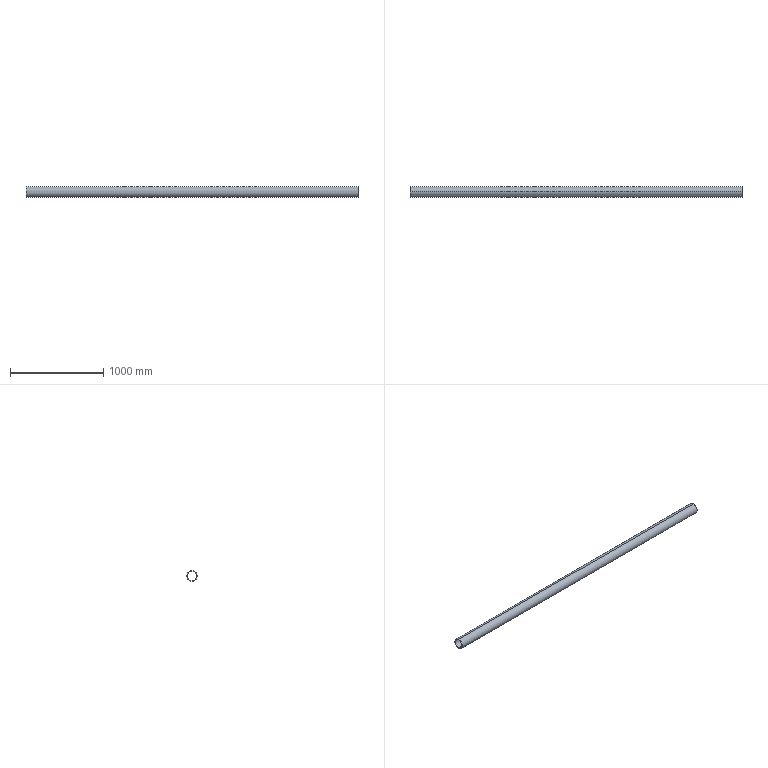Part | STEP file | Input 31 | 1 solid | 6 faces | box 3557 x 114.3 x 114.3 mm | volume 7284143 mm3 | cylinder 4 | plane 2 | commonest cylinder face diameters 102.26 x2 114.3 x2
STEP:
#1=CARTESIAN_POINT('',(0.,0.,0.));
#2=DIRECTION('',(0.,0.,1.));
#3=DIRECTION('',(1.,0.,0.));
#4=AXIS2_PLACEMENT_3D('',#1,#2,#3);
#5=CARTESIAN_POINT('',(117.,0.09044,51.13));
#6=VERTEX_POINT('',#5);
#7=CARTESIAN_POINT('',(-3440.,0.09044,51.13));
#8=VERTEX_POINT('',#7);
#9=CARTESIAN_POINT('',(117.,0.09044,51.13));
#10=DIRECTION('',(-1.,0.,0.));
#11=VECTOR('',#10,1.);
#12=LINE('',#9,#11);
#13=CARTESIAN_POINT('',(117.,0.,0.));
#14=DIRECTION('',(-1.,0.,0.));
#15=DIRECTION('',(0.,0.001769,1.));
#16=AXIS2_PLACEMENT_3D('',#13,#14,#15);
#17=CYLINDRICAL_SURFACE('',#16,51.13);
#18=CARTESIAN_POINT('',(6.283,0.));
#19=DIRECTION('',(0.,1.));
#20=VECTOR('',#19,1.);
#21=LINE('',#18,#20);
#22=(GEOMETRIC_REPRESENTATION_CONTEXT(2)PARAMETRIC_REPRESENTATION_CONTEXT()REPRESENTATION_CONTEXT('',''));
#23=DEFINITIONAL_REPRESENTATION('',(#21),#22);
#24=PCURVE('',#17,#23);
#25=CARTESIAN_POINT('',(117.,0.,0.));
#26=DIRECTION('',(-1.,0.,0.));
#27=DIRECTION('',(0.,0.001769,1.));
#28=AXIS2_PLACEMENT_3D('',#25,#26,#27);
#29=CYLINDRICAL_SURFACE('',#28,51.13);
#30=CARTESIAN_POINT('',(0.,0.));
#31=DIRECTION('',(0.,1.));
#32=VECTOR('',#31,1.);
#33=LINE('',#30,#32);
#34=(GEOMETRIC_REPRESENTATION_CONTEXT(2)PARAMETRIC_REPRESENTATION_CONTEXT()REPRESENTATION_CONTEXT('',''));
#35=DEFINITIONAL_REPRESENTATION('',(#33),#34);
#36=PCURVE('',#29,#35);
#37=SURFACE_CURVE('',#12,(#24,#36),.PCURVE_S1.);
#38=EDGE_CURVE('',#6,#8,#37,.T.);
#39=ORIENTED_EDGE('',*,*,#38,.T.);
#40=CARTESIAN_POINT('',(-3440.,-0.09044,-51.13));
#41=VERTEX_POINT('',#40);
#42=CARTESIAN_POINT('',(-3440.,0.,0.));
#43=DIRECTION('',(-1.,0.,0.));
#44=DIRECTION('',(0.,0.001769,1.));
#45=AXIS2_PLACEMENT_3D('',#42,#43,#44);
#46=CIRCLE('',#45,51.13);
#47=CARTESIAN_POINT('',(0.,3557.));
#48=DIRECTION('',(1.,0.));
#49=VECTOR('',#48,1.);
#50=LINE('',#47,#49);
#51=(GEOMETRIC_REPRESENTATION_CONTEXT(2)PARAMETRIC_REPRESENTATION_CONTEXT()REPRESENTATION_CONTEXT('',''));
#52=DEFINITIONAL_REPRESENTATION('',(#50),#51);
#53=PCURVE('',#17,#52);
#54=CARTESIAN_POINT('',(-3440.,0.,0.));
#55=DIRECTION('',(-1.,0.,0.));
#56=DIRECTION('',(0.,0.001769,1.));
#57=AXIS2_PLACEMENT_3D('',#54,#55,#56);
#58=PLANE('',#57);
#59=CARTESIAN_POINT('',(0.,0.));
#60=DIRECTION('',(1.,0.));
#61=AXIS2_PLACEMENT_2D('',#59,#60);
#62=CIRCLE('',#61,51.13);
#63=(GEOMETRIC_REPRESENTATION_CONTEXT(2)PARAMETRIC_REPRESENTATION_CONTEXT()REPRESENTATION_CONTEXT('',''));
#64=DEFINITIONAL_REPRESENTATION('',(#62),#63);
#65=PCURVE('',#58,#64);
#66=SURFACE_CURVE('',#46,(#53,#65),.PCURVE_S1.);
#67=EDGE_CURVE('',#41,#8,#66,.T.);
#68=ORIENTED_EDGE('',*,*,#67,.F.);
#69=CARTESIAN_POINT('',(117.,-0.09044,-51.13));
#70=VERTEX_POINT('',#69);
#71=CARTESIAN_POINT('',(117.,-0.09044,-51.13));
#72=DIRECTION('',(-1.,0.,0.));
#73=VECTOR('',#72,1.);
#74=LINE('',#71,#73);
#75=CARTESIAN_POINT('',(3.142,0.));
#76=DIRECTION('',(0.,1.));
#77=VECTOR('',#76,1.);
#78=LINE('',#75,#77);
#79=(GEOMETRIC_REPRESENTATION_CONTEXT(2)PARAMETRIC_REPRESENTATION_CONTEXT()REPRESENTATION_CONTEXT('',''));
#80=DEFINITIONAL_REPRESENTATION('',(#78),#79);
#81=PCURVE('',#17,#80);
#82=CARTESIAN_POINT('',(3.142,0.));
#83=DIRECTION('',(0.,1.));
#84=VECTOR('',#83,1.);
#85=LINE('',#82,#84);
#86=(GEOMETRIC_REPRESENTATION_CONTEXT(2)PARAMETRIC_REPRESENTATION_CONTEXT()REPRESENTATION_CONTEXT('',''));
#87=DEFINITIONAL_REPRESENTATION('',(#85),#86);
#88=PCURVE('',#29,#87);
#89=SURFACE_CURVE('',#74,(#81,#88),.PCURVE_S1.);
#90=EDGE_CURVE('',#70,#41,#89,.T.);
#91=ORIENTED_EDGE('',*,*,#90,.F.);
#92=CARTESIAN_POINT('',(117.,0.,0.));
#93=DIRECTION('',(-1.,0.,0.));
#94=DIRECTION('',(0.,0.001769,1.));
#95=AXIS2_PLACEMENT_3D('',#92,#93,#94);
#96=CIRCLE('',#95,51.13);
#97=CARTESIAN_POINT('',(0.,0.));
#98=DIRECTION('',(1.,0.));
#99=VECTOR('',#98,1.);
#100=LINE('',#97,#99);
#101=(GEOMETRIC_REPRESENTATION_CONTEXT(2)PARAMETRIC_REPRESENTATION_CONTEXT()REPRESENTATION_CONTEXT('',''));
#102=DEFINITIONAL_REPRESENTATION('',(#100),#101);
#103=PCURVE('',#17,#102);
#104=CARTESIAN_POINT('',(117.,0.,0.));
#105=DIRECTION('',(-1.,0.,0.));
#106=DIRECTION('',(0.,0.001769,1.));
#107=AXIS2_PLACEMENT_3D('',#104,#105,#106);
#108=PLANE('',#107);
#109=CARTESIAN_POINT('',(0.,0.));
#110=DIRECTION('',(1.,0.));
#111=AXIS2_PLACEMENT_2D('',#109,#110);
#112=CIRCLE('',#111,51.13);
#113=(GEOMETRIC_REPRESENTATION_CONTEXT(2)PARAMETRIC_REPRESENTATION_CONTEXT()REPRESENTATION_CONTEXT('',''));
#114=DEFINITIONAL_REPRESENTATION('',(#112),#113);
#115=PCURVE('',#108,#114);
#116=SURFACE_CURVE('',#96,(#103,#115),.PCURVE_S1.);
#117=EDGE_CURVE('',#70,#6,#116,.T.);
#118=ORIENTED_EDGE('',*,*,#117,.T.);
#119=EDGE_LOOP('',(#39,#68,#91,#118));
#120=FACE_BOUND('',#119,.F.);
#121=ADVANCED_FACE('',(#120),#17,.F.);
#122=CARTESIAN_POINT('',(117.,0.1011,57.15));
#123=VERTEX_POINT('',#122);
#124=CARTESIAN_POINT('',(117.,-0.1011,-57.15));
#125=VERTEX_POINT('',#124);
#126=CARTESIAN_POINT('',(117.,0.,0.));
#127=DIRECTION('',(-1.,0.,0.));
#128=DIRECTION('',(0.,0.001769,1.));
#129=AXIS2_PLACEMENT_3D('',#126,#127,#128);
#130=CIRCLE('',#129,57.15);
#131=CARTESIAN_POINT('',(117.,0.,0.));
#132=DIRECTION('',(-1.,0.,0.));
#133=DIRECTION('',(0.,0.001769,1.));
#134=AXIS2_PLACEMENT_3D('',#131,#132,#133);
#135=CYLINDRICAL_SURFACE('',#134,57.15);
#136=CARTESIAN_POINT('',(0.,0.));
#137=DIRECTION('',(1.,0.));
#138=VECTOR('',#137,1.);
#139=LINE('',#136,#138);
#140=(GEOMETRIC_REPRESENTATION_CONTEXT(2)PARAMETRIC_REPRESENTATION_CONTEXT()REPRESENTATION_CONTEXT('',''));
#141=DEFINITIONAL_REPRESENTATION('',(#139),#140);
#142=PCURVE('',#135,#141);
#143=CARTESIAN_POINT('',(0.,0.));
#144=DIRECTION('',(1.,0.));
#145=AXIS2_PLACEMENT_2D('',#143,#144);
#146=CIRCLE('',#145,57.15);
#147=(GEOMETRIC_REPRESENTATION_CONTEXT(2)PARAMETRIC_REPRESENTATION_CONTEXT()REPRESENTATION_CONTEXT('',''));
#148=DEFINITIONAL_REPRESENTATION('',(#146),#147);
#149=PCURVE('',#108,#148);
#150=SURFACE_CURVE('',#130,(#142,#149),.PCURVE_S1.);
#151=EDGE_CURVE('',#123,#125,#150,.T.);
#152=ORIENTED_EDGE('',*,*,#151,.T.);
#153=CARTESIAN_POINT('',(-3440.,-0.1011,-57.15));
#154=VERTEX_POINT('',#153);
#155=CARTESIAN_POINT('',(117.,-0.1011,-57.15));
#156=DIRECTION('',(-1.,0.,0.));
#157=VECTOR('',#156,1.);
#158=LINE('',#155,#157);
#159=CARTESIAN_POINT('',(3.142,0.));
#160=DIRECTION('',(0.,1.));
#161=VECTOR('',#160,1.);
#162=LINE('',#159,#161);
#163=(GEOMETRIC_REPRESENTATION_CONTEXT(2)PARAMETRIC_REPRESENTATION_CONTEXT()REPRESENTATION_CONTEXT('',''));
#164=DEFINITIONAL_REPRESENTATION('',(#162),#163);
#165=PCURVE('',#135,#164);
#166=CARTESIAN_POINT('',(117.,0.,0.));
#167=DIRECTION('',(-1.,0.,0.));
#168=DIRECTION('',(0.,0.001769,1.));
#169=AXIS2_PLACEMENT_3D('',#166,#167,#168);
#170=CYLINDRICAL_SURFACE('',#169,57.15);
#171=CARTESIAN_POINT('',(3.142,0.));
#172=DIRECTION('',(0.,1.));
#173=VECTOR('',#172,1.);
#174=LINE('',#171,#173);
#175=(GEOMETRIC_REPRESENTATION_CONTEXT(2)PARAMETRIC_REPRESENTATION_CONTEXT()REPRESENTATION_CONTEXT('',''));
#176=DEFINITIONAL_REPRESENTATION('',(#174),#175);
#177=PCURVE('',#170,#176);
#178=SURFACE_CURVE('',#158,(#165,#177),.PCURVE_S1.);
#179=EDGE_CURVE('',#125,#154,#178,.T.);
#180=ORIENTED_EDGE('',*,*,#179,.T.);
#181=CARTESIAN_POINT('',(-3440.,0.1011,57.15));
#182=VERTEX_POINT('',#181);
#183=CARTESIAN_POINT('',(-3440.,0.,0.));
#184=DIRECTION('',(-1.,0.,0.));
#185=DIRECTION('',(0.,0.001769,1.));
#186=AXIS2_PLACEMENT_3D('',#183,#184,#185);
#187=CIRCLE('',#186,57.15);
#188=CARTESIAN_POINT('',(0.,3557.));
#189=DIRECTION('',(1.,0.));
#190=VECTOR('',#189,1.);
#191=LINE('',#188,#190);
#192=(GEOMETRIC_REPRESENTATION_CONTEXT(2)PARAMETRIC_REPRESENTATION_CONTEXT()REPRESENTATION_CONTEXT('',''));
#193=DEFINITIONAL_REPRESENTATION('',(#191),#192);
#194=PCURVE('',#135,#193);
#195=CARTESIAN_POINT('',(0.,0.));
#196=DIRECTION('',(1.,0.));
#197=AXIS2_PLACEMENT_2D('',#195,#196);
#198=CIRCLE('',#197,57.15);
#199=(GEOMETRIC_REPRESENTATION_CONTEXT(2)PARAMETRIC_REPRESENTATION_CONTEXT()REPRESENTATION_CONTEXT('',''));
#200=DEFINITIONAL_REPRESENTATION('',(#198),#199);
#201=PCURVE('',#58,#200);
#202=SURFACE_CURVE('',#187,(#194,#201),.PCURVE_S1.);
#203=EDGE_CURVE('',#182,#154,#202,.T.);
#204=ORIENTED_EDGE('',*,*,#203,.F.);
#205=CARTESIAN_POINT('',(117.,0.1011,57.15));
#206=DIRECTION('',(-1.,0.,0.));
#207=VECTOR('',#206,1.);
#208=LINE('',#205,#207);
#209=CARTESIAN_POINT('',(0.,0.));
#210=DIRECTION('',(0.,1.));
#211=VECTOR('',#210,1.);
#212=LINE('',#209,#211);
#213=(GEOMETRIC_REPRESENTATION_CONTEXT(2)PARAMETRIC_REPRESENTATION_CONTEXT()REPRESENTATION_CONTEXT('',''));
#214=DEFINITIONAL_REPRESENTATION('',(#212),#213);
#215=PCURVE('',#135,#214);
#216=CARTESIAN_POINT('',(6.283,0.));
#217=DIRECTION('',(0.,1.));
#218=VECTOR('',#217,1.);
#219=LINE('',#216,#218);
#220=(GEOMETRIC_REPRESENTATION_CONTEXT(2)PARAMETRIC_REPRESENTATION_CONTEXT()REPRESENTATION_CONTEXT('',''));
#221=DEFINITIONAL_REPRESENTATION('',(#219),#220);
#222=PCURVE('',#170,#221);
#223=SURFACE_CURVE('',#208,(#215,#222),.PCURVE_S1.);
#224=EDGE_CURVE('',#123,#182,#223,.T.);
#225=ORIENTED_EDGE('',*,*,#224,.F.);
#226=EDGE_LOOP('',(#152,#180,#204,#225));
#227=FACE_BOUND('',#226,.T.);
#228=ADVANCED_FACE('',(#227),#135,.T.);
#229=ORIENTED_EDGE('',*,*,#179,.F.);
#230=CARTESIAN_POINT('',(117.,0.,0.));
#231=DIRECTION('',(-1.,0.,0.));
#232=DIRECTION('',(0.,0.001769,1.));
#233=AXIS2_PLACEMENT_3D('',#230,#231,#232);
#234=CIRCLE('',#233,57.15);
#235=CARTESIAN_POINT('',(0.,0.));
#236=DIRECTION('',(1.,0.));
#237=VECTOR('',#236,1.);
#238=LINE('',#235,#237);
#239=(GEOMETRIC_REPRESENTATION_CONTEXT(2)PARAMETRIC_REPRESENTATION_CONTEXT()REPRESENTATION_CONTEXT('',''));
#240=DEFINITIONAL_REPRESENTATION('',(#238),#239);
#241=PCURVE('',#170,#240);
#242=CARTESIAN_POINT('',(0.,0.));
#243=DIRECTION('',(1.,0.));
#244=AXIS2_PLACEMENT_2D('',#242,#243);
#245=CIRCLE('',#244,57.15);
#246=(GEOMETRIC_REPRESENTATION_CONTEXT(2)PARAMETRIC_REPRESENTATION_CONTEXT()REPRESENTATION_CONTEXT('',''));
#247=DEFINITIONAL_REPRESENTATION('',(#245),#246);
#248=PCURVE('',#108,#247);
#249=SURFACE_CURVE('',#234,(#241,#248),.PCURVE_S1.);
#250=EDGE_CURVE('',#125,#123,#249,.T.);
#251=ORIENTED_EDGE('',*,*,#250,.T.);
#252=ORIENTED_EDGE('',*,*,#224,.T.);
#253=CARTESIAN_POINT('',(-3440.,0.,0.));
#254=DIRECTION('',(-1.,0.,0.));
#255=DIRECTION('',(0.,0.001769,1.));
#256=AXIS2_PLACEMENT_3D('',#253,#254,#255);
#257=CIRCLE('',#256,57.15);
#258=CARTESIAN_POINT('',(0.,3557.));
#259=DIRECTION('',(1.,0.));
#260=VECTOR('',#259,1.);
#261=LINE('',#258,#260);
#262=(GEOMETRIC_REPRESENTATION_CONTEXT(2)PARAMETRIC_REPRESENTATION_CONTEXT()REPRESENTATION_CONTEXT('',''));
#263=DEFINITIONAL_REPRESENTATION('',(#261),#262);
#264=PCURVE('',#170,#263);
#265=CARTESIAN_POINT('',(0.,0.));
#266=DIRECTION('',(1.,0.));
#267=AXIS2_PLACEMENT_2D('',#265,#266);
#268=CIRCLE('',#267,57.15);
#269=(GEOMETRIC_REPRESENTATION_CONTEXT(2)PARAMETRIC_REPRESENTATION_CONTEXT()REPRESENTATION_CONTEXT('',''));
#270=DEFINITIONAL_REPRESENTATION('',(#268),#269);
#271=PCURVE('',#58,#270);
#272=SURFACE_CURVE('',#257,(#264,#271),.PCURVE_S1.);
#273=EDGE_CURVE('',#154,#182,#272,.T.);
#274=ORIENTED_EDGE('',*,*,#273,.F.);
#275=EDGE_LOOP('',(#229,#251,#252,#274));
#276=FACE_BOUND('',#275,.T.);
#277=ADVANCED_FACE('',(#276),#170,.T.);
#278=CARTESIAN_POINT('',(117.,0.,0.));
#279=DIRECTION('',(-1.,0.,0.));
#280=DIRECTION('',(0.,0.001769,1.));
#281=AXIS2_PLACEMENT_3D('',#278,#279,#280);
#282=CIRCLE('',#281,51.13);
#283=CARTESIAN_POINT('',(0.,0.));
#284=DIRECTION('',(1.,0.));
#285=AXIS2_PLACEMENT_2D('',#283,#284);
#286=CIRCLE('',#285,51.13);
#287=(GEOMETRIC_REPRESENTATION_CONTEXT(2)PARAMETRIC_REPRESENTATION_CONTEXT()REPRESENTATION_CONTEXT('',''));
#288=DEFINITIONAL_REPRESENTATION('',(#286),#287);
#289=PCURVE('',#108,#288);
#290=CARTESIAN_POINT('',(0.,0.));
#291=DIRECTION('',(1.,0.));
#292=VECTOR('',#291,1.);
#293=LINE('',#290,#292);
#294=(GEOMETRIC_REPRESENTATION_CONTEXT(2)PARAMETRIC_REPRESENTATION_CONTEXT()REPRESENTATION_CONTEXT('',''));
#295=DEFINITIONAL_REPRESENTATION('',(#293),#294);
#296=PCURVE('',#29,#295);
#297=SURFACE_CURVE('',#282,(#289,#296),.PCURVE_S1.);
#298=EDGE_CURVE('',#6,#70,#297,.T.);
#299=ORIENTED_EDGE('',*,*,#298,.T.);
#300=ORIENTED_EDGE('',*,*,#117,.T.);
#301=EDGE_LOOP('',(#299,#300));
#302=FACE_BOUND('',#301,.T.);
#303=ORIENTED_EDGE('',*,*,#151,.F.);
#304=ORIENTED_EDGE('',*,*,#250,.F.);
#305=EDGE_LOOP('',(#303,#304));
#306=FACE_BOUND('',#305,.T.);
#307=ADVANCED_FACE('',(#302,#306),#108,.F.);
#308=CARTESIAN_POINT('',(-3440.,0.,0.));
#309=DIRECTION('',(-1.,0.,0.));
#310=DIRECTION('',(0.,0.001769,1.));
#311=AXIS2_PLACEMENT_3D('',#308,#309,#310);
#312=CIRCLE('',#311,51.13);
#313=CARTESIAN_POINT('',(0.,0.));
#314=DIRECTION('',(1.,0.));
#315=AXIS2_PLACEMENT_2D('',#313,#314);
#316=CIRCLE('',#315,51.13);
#317=(GEOMETRIC_REPRESENTATION_CONTEXT(2)PARAMETRIC_REPRESENTATION_CONTEXT()REPRESENTATION_CONTEXT('',''));
#318=DEFINITIONAL_REPRESENTATION('',(#316),#317);
#319=PCURVE('',#58,#318);
#320=CARTESIAN_POINT('',(0.,3557.));
#321=DIRECTION('',(1.,0.));
#322=VECTOR('',#321,1.);
#323=LINE('',#320,#322);
#324=(GEOMETRIC_REPRESENTATION_CONTEXT(2)PARAMETRIC_REPRESENTATION_CONTEXT()REPRESENTATION_CONTEXT('',''));
#325=DEFINITIONAL_REPRESENTATION('',(#323),#324);
#326=PCURVE('',#29,#325);
#327=SURFACE_CURVE('',#312,(#319,#326),.PCURVE_S1.);
#328=EDGE_CURVE('',#8,#41,#327,.T.);
#329=ORIENTED_EDGE('',*,*,#328,.F.);
#330=ORIENTED_EDGE('',*,*,#67,.F.);
#331=EDGE_LOOP('',(#329,#330));
#332=FACE_BOUND('',#331,.T.);
#333=ORIENTED_EDGE('',*,*,#203,.T.);
#334=ORIENTED_EDGE('',*,*,#273,.T.);
#335=EDGE_LOOP('',(#333,#334));
#336=FACE_BOUND('',#335,.T.);
#337=ADVANCED_FACE('',(#332,#336),#58,.T.);
#338=ORIENTED_EDGE('',*,*,#328,.F.);
#339=ORIENTED_EDGE('',*,*,#38,.F.);
#340=ORIENTED_EDGE('',*,*,#298,.T.);
#341=ORIENTED_EDGE('',*,*,#90,.T.);
#342=EDGE_LOOP('',(#338,#339,#340,#341));
#343=FACE_BOUND('',#342,.F.);
#344=ADVANCED_FACE('',(#343),#29,.F.);
#345=CLOSED_SHELL('',(#121,#228,#277,#307,#337,#344));
#346=MANIFOLD_SOLID_BREP('',#345);
#347=(LENGTH_UNIT()NAMED_UNIT(*)SI_UNIT(.MILLI.,.METRE.));
#348=UNCERTAINTY_MEASURE_WITH_UNIT(LENGTH_MEASURE(0.0000001),#347,'','');
#349=(NAMED_UNIT(*)PLANE_ANGLE_UNIT()SI_UNIT($,.RADIAN.));
#350=(NAMED_UNIT(*)SI_UNIT($,.STERADIAN.)SOLID_ANGLE_UNIT());
#351=(GEOMETRIC_REPRESENTATION_CONTEXT(3)GLOBAL_UNCERTAINTY_ASSIGNED_CONTEXT((#348))GLOBAL_UNIT_ASSIGNED_CONTEXT((#347,#349,#350))REPRESENTATION_CONTEXT('',''));
#352=ADVANCED_BREP_SHAPE_REPRESENTATION('',(#4,#346),#351);